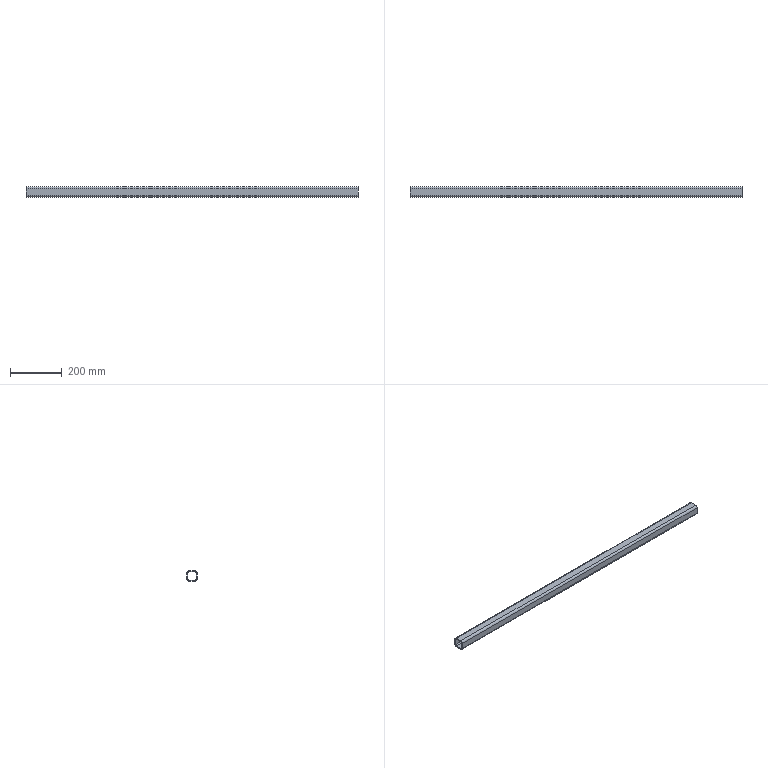Part | SolidWorks | features WeldMemberFeat 1, WeldmentFeature 1 | 1 solid | 18 faces | box 1280 x 40 x 40 mm | volume 684539 mm3 | plane 10 | cylinder 8 | commonest cylinder face diameters 8 x4 16 x4
STEP:
#1=CARTESIAN_POINT('',(-1000.,20.,12.));
#2=VERTEX_POINT('',#1);
#3=CARTESIAN_POINT('',(-1000.,12.,20.));
#4=VERTEX_POINT('',#3);
#5=CARTESIAN_POINT('',(-1000.,12.,12.));
#6=DIRECTION('',(1.,0.,0.));
#7=DIRECTION('',(0.,0.,-1.));
#8=AXIS2_PLACEMENT_3D('',#5,#6,#7);
#9=CIRCLE('',#8,8.);
#10=EDGE_CURVE('',#2,#4,#9,.T.);
#11=ORIENTED_EDGE('',*,*,#10,.T.);
#12=CARTESIAN_POINT('',(280.,12.,20.));
#13=VERTEX_POINT('',#12);
#14=CARTESIAN_POINT('',(280.,12.,20.));
#15=DIRECTION('',(-1.,0.,0.));
#16=VECTOR('',#15,1000.);
#17=LINE('',#14,#16);
#18=EDGE_CURVE('',#13,#4,#17,.T.);
#19=ORIENTED_EDGE('',*,*,#18,.F.);
#20=CARTESIAN_POINT('',(280.,20.,12.));
#21=VERTEX_POINT('',#20);
#22=CARTESIAN_POINT('',(280.,12.,12.));
#23=DIRECTION('',(1.,0.,0.));
#24=DIRECTION('',(0.,0.,-1.));
#25=AXIS2_PLACEMENT_3D('',#22,#23,#24);
#26=CIRCLE('',#25,8.);
#27=EDGE_CURVE('',#21,#13,#26,.T.);
#28=ORIENTED_EDGE('',*,*,#27,.F.);
#29=CARTESIAN_POINT('',(280.,20.,12.));
#30=DIRECTION('',(-1.,0.,0.));
#31=VECTOR('',#30,1000.);
#32=LINE('',#29,#31);
#33=EDGE_CURVE('',#21,#2,#32,.T.);
#34=ORIENTED_EDGE('',*,*,#33,.T.);
#35=EDGE_LOOP('',(#11,#19,#28,#34));
#36=FACE_OUTER_BOUND('',#35,.T.);
#37=CARTESIAN_POINT('',(280.,12.,12.));
#38=DIRECTION('',(-1.,0.,0.));
#39=DIRECTION('',(0.,0.,1.));
#40=AXIS2_PLACEMENT_3D('',#37,#38,#39);
#41=CYLINDRICAL_SURFACE('',#40,8.);
#42=ADVANCED_FACE('',(#36),#41,.T.);
#43=CARTESIAN_POINT('',(-1000.,-12.,20.));
#44=VERTEX_POINT('',#43);
#45=CARTESIAN_POINT('',(-1000.,12.,20.));
#46=DIRECTION('',(0.,-1.,0.));
#47=VECTOR('',#46,1000.);
#48=LINE('',#45,#47);
#49=EDGE_CURVE('',#4,#44,#48,.T.);
#50=ORIENTED_EDGE('',*,*,#49,.T.);
#51=CARTESIAN_POINT('',(280.,-12.,20.));
#52=VERTEX_POINT('',#51);
#53=CARTESIAN_POINT('',(280.,-12.,20.));
#54=DIRECTION('',(-1.,0.,0.));
#55=VECTOR('',#54,1000.);
#56=LINE('',#53,#55);
#57=EDGE_CURVE('',#52,#44,#56,.T.);
#58=ORIENTED_EDGE('',*,*,#57,.F.);
#59=CARTESIAN_POINT('',(280.,12.,20.));
#60=DIRECTION('',(0.,-1.,0.));
#61=VECTOR('',#60,1000.);
#62=LINE('',#59,#61);
#63=EDGE_CURVE('',#13,#52,#62,.T.);
#64=ORIENTED_EDGE('',*,*,#63,.F.);
#65=ORIENTED_EDGE('',*,*,#18,.T.);
#66=EDGE_LOOP('',(#50,#58,#64,#65));
#67=FACE_OUTER_BOUND('',#66,.T.);
#68=CARTESIAN_POINT('',(280.,12.,20.));
#69=DIRECTION('',(0.,0.,-1.));
#70=DIRECTION('',(-1.,0.,0.));
#71=AXIS2_PLACEMENT_3D('',#68,#69,#70);
#72=PLANE('',#71);
#73=ADVANCED_FACE('',(#67),#72,.F.);
#74=CARTESIAN_POINT('',(-1000.,-20.,12.));
#75=VERTEX_POINT('',#74);
#76=CARTESIAN_POINT('',(-1000.,-12.,12.));
#77=DIRECTION('',(1.,0.,0.));
#78=DIRECTION('',(0.,0.,-1.));
#79=AXIS2_PLACEMENT_3D('',#76,#77,#78);
#80=CIRCLE('',#79,8.);
#81=EDGE_CURVE('',#44,#75,#80,.T.);
#82=ORIENTED_EDGE('',*,*,#81,.T.);
#83=CARTESIAN_POINT('',(280.,-20.,12.));
#84=VERTEX_POINT('',#83);
#85=CARTESIAN_POINT('',(280.,-20.,12.));
#86=DIRECTION('',(-1.,0.,0.));
#87=VECTOR('',#86,1000.);
#88=LINE('',#85,#87);
#89=EDGE_CURVE('',#84,#75,#88,.T.);
#90=ORIENTED_EDGE('',*,*,#89,.F.);
#91=CARTESIAN_POINT('',(280.,-12.,12.));
#92=DIRECTION('',(1.,0.,0.));
#93=DIRECTION('',(0.,0.,-1.));
#94=AXIS2_PLACEMENT_3D('',#91,#92,#93);
#95=CIRCLE('',#94,8.);
#96=EDGE_CURVE('',#52,#84,#95,.T.);
#97=ORIENTED_EDGE('',*,*,#96,.F.);
#98=ORIENTED_EDGE('',*,*,#57,.T.);
#99=EDGE_LOOP('',(#82,#90,#97,#98));
#100=FACE_OUTER_BOUND('',#99,.T.);
#101=CARTESIAN_POINT('',(280.,-12.,12.));
#102=DIRECTION('',(-1.,0.,0.));
#103=DIRECTION('',(0.,0.,1.));
#104=AXIS2_PLACEMENT_3D('',#101,#102,#103);
#105=CYLINDRICAL_SURFACE('',#104,8.);
#106=ADVANCED_FACE('',(#100),#105,.T.);
#107=CARTESIAN_POINT('',(-1000.,-20.,-12.));
#108=VERTEX_POINT('',#107);
#109=CARTESIAN_POINT('',(-1000.,-20.,-12.));
#110=DIRECTION('',(0.,0.,-1.));
#111=VECTOR('',#110,1000.);
#112=LINE('',#109,#111);
#113=EDGE_CURVE('',#75,#108,#112,.T.);
#114=ORIENTED_EDGE('',*,*,#113,.T.);
#115=CARTESIAN_POINT('',(280.,-20.,-12.));
#116=VERTEX_POINT('',#115);
#117=CARTESIAN_POINT('',(280.,-20.,-12.));
#118=DIRECTION('',(-1.,0.,0.));
#119=VECTOR('',#118,1000.);
#120=LINE('',#117,#119);
#121=EDGE_CURVE('',#116,#108,#120,.T.);
#122=ORIENTED_EDGE('',*,*,#121,.F.);
#123=CARTESIAN_POINT('',(280.,-20.,-12.));
#124=DIRECTION('',(0.,0.,-1.));
#125=VECTOR('',#124,1000.);
#126=LINE('',#123,#125);
#127=EDGE_CURVE('',#84,#116,#126,.T.);
#128=ORIENTED_EDGE('',*,*,#127,.F.);
#129=ORIENTED_EDGE('',*,*,#89,.T.);
#130=EDGE_LOOP('',(#114,#122,#128,#129));
#131=FACE_OUTER_BOUND('',#130,.T.);
#132=CARTESIAN_POINT('',(280.,-20.,-12.));
#133=DIRECTION('',(0.,1.,0.));
#134=DIRECTION('',(0.,0.,1.));
#135=AXIS2_PLACEMENT_3D('',#132,#133,#134);
#136=PLANE('',#135);
#137=ADVANCED_FACE('',(#131),#136,.F.);
#138=CARTESIAN_POINT('',(-1000.,-12.,-20.));
#139=VERTEX_POINT('',#138);
#140=CARTESIAN_POINT('',(-1000.,-12.,-12.));
#141=DIRECTION('',(1.,0.,0.));
#142=DIRECTION('',(0.,0.,-1.));
#143=AXIS2_PLACEMENT_3D('',#140,#141,#142);
#144=CIRCLE('',#143,8.);
#145=EDGE_CURVE('',#108,#139,#144,.T.);
#146=ORIENTED_EDGE('',*,*,#145,.T.);
#147=CARTESIAN_POINT('',(280.,-12.,-20.));
#148=VERTEX_POINT('',#147);
#149=CARTESIAN_POINT('',(280.,-12.,-20.));
#150=DIRECTION('',(-1.,0.,0.));
#151=VECTOR('',#150,1000.);
#152=LINE('',#149,#151);
#153=EDGE_CURVE('',#148,#139,#152,.T.);
#154=ORIENTED_EDGE('',*,*,#153,.F.);
#155=CARTESIAN_POINT('',(280.,-12.,-12.));
#156=DIRECTION('',(1.,0.,0.));
#157=DIRECTION('',(0.,0.,-1.));
#158=AXIS2_PLACEMENT_3D('',#155,#156,#157);
#159=CIRCLE('',#158,8.);
#160=EDGE_CURVE('',#116,#148,#159,.T.);
#161=ORIENTED_EDGE('',*,*,#160,.F.);
#162=ORIENTED_EDGE('',*,*,#121,.T.);
#163=EDGE_LOOP('',(#146,#154,#161,#162));
#164=FACE_OUTER_BOUND('',#163,.T.);
#165=CARTESIAN_POINT('',(280.,-12.,-12.));
#166=DIRECTION('',(-1.,0.,0.));
#167=DIRECTION('',(0.,0.,1.));
#168=AXIS2_PLACEMENT_3D('',#165,#166,#167);
#169=CYLINDRICAL_SURFACE('',#168,8.);
#170=ADVANCED_FACE('',(#164),#169,.T.);
#171=CARTESIAN_POINT('',(-1000.,12.,-20.));
#172=VERTEX_POINT('',#171);
#173=CARTESIAN_POINT('',(-1000.,-12.,-20.));
#174=DIRECTION('',(0.,1.,0.));
#175=VECTOR('',#174,1000.);
#176=LINE('',#173,#175);
#177=EDGE_CURVE('',#139,#172,#176,.T.);
#178=ORIENTED_EDGE('',*,*,#177,.T.);
#179=CARTESIAN_POINT('',(280.,12.,-20.));
#180=VERTEX_POINT('',#179);
#181=CARTESIAN_POINT('',(280.,12.,-20.));
#182=DIRECTION('',(-1.,0.,0.));
#183=VECTOR('',#182,1000.);
#184=LINE('',#181,#183);
#185=EDGE_CURVE('',#180,#172,#184,.T.);
#186=ORIENTED_EDGE('',*,*,#185,.F.);
#187=CARTESIAN_POINT('',(280.,-12.,-20.));
#188=DIRECTION('',(0.,1.,0.));
#189=VECTOR('',#188,1000.);
#190=LINE('',#187,#189);
#191=EDGE_CURVE('',#148,#180,#190,.T.);
#192=ORIENTED_EDGE('',*,*,#191,.F.);
#193=ORIENTED_EDGE('',*,*,#153,.T.);
#194=EDGE_LOOP('',(#178,#186,#192,#193));
#195=FACE_OUTER_BOUND('',#194,.T.);
#196=CARTESIAN_POINT('',(280.,-12.,-20.));
#197=DIRECTION('',(0.,0.,1.));
#198=DIRECTION('',(1.,0.,0.));
#199=AXIS2_PLACEMENT_3D('',#196,#197,#198);
#200=PLANE('',#199);
#201=ADVANCED_FACE('',(#195),#200,.F.);
#202=CARTESIAN_POINT('',(-1000.,20.,-12.));
#203=VERTEX_POINT('',#202);
#204=CARTESIAN_POINT('',(-1000.,12.,-12.));
#205=DIRECTION('',(1.,0.,0.));
#206=DIRECTION('',(0.,0.,-1.));
#207=AXIS2_PLACEMENT_3D('',#204,#205,#206);
#208=CIRCLE('',#207,8.);
#209=EDGE_CURVE('',#172,#203,#208,.T.);
#210=ORIENTED_EDGE('',*,*,#209,.T.);
#211=CARTESIAN_POINT('',(280.,20.,-12.));
#212=VERTEX_POINT('',#211);
#213=CARTESIAN_POINT('',(280.,20.,-12.));
#214=DIRECTION('',(-1.,0.,0.));
#215=VECTOR('',#214,1000.);
#216=LINE('',#213,#215);
#217=EDGE_CURVE('',#212,#203,#216,.T.);
#218=ORIENTED_EDGE('',*,*,#217,.F.);
#219=CARTESIAN_POINT('',(280.,12.,-12.));
#220=DIRECTION('',(1.,0.,0.));
#221=DIRECTION('',(0.,0.,-1.));
#222=AXIS2_PLACEMENT_3D('',#219,#220,#221);
#223=CIRCLE('',#222,8.);
#224=EDGE_CURVE('',#180,#212,#223,.T.);
#225=ORIENTED_EDGE('',*,*,#224,.F.);
#226=ORIENTED_EDGE('',*,*,#185,.T.);
#227=EDGE_LOOP('',(#210,#218,#225,#226));
#228=FACE_OUTER_BOUND('',#227,.T.);
#229=CARTESIAN_POINT('',(280.,12.,-12.));
#230=DIRECTION('',(-1.,0.,0.));
#231=DIRECTION('',(0.,0.,1.));
#232=AXIS2_PLACEMENT_3D('',#229,#230,#231);
#233=CYLINDRICAL_SURFACE('',#232,8.);
#234=ADVANCED_FACE('',(#228),#233,.T.);
#235=CARTESIAN_POINT('',(-1000.,-12.,16.));
#236=VERTEX_POINT('',#235);
#237=CARTESIAN_POINT('',(-1000.,-16.,12.));
#238=VERTEX_POINT('',#237);
#239=CARTESIAN_POINT('',(-1000.,-12.,12.));
#240=DIRECTION('',(1.,0.,0.));
#241=DIRECTION('',(0.,0.,-1.));
#242=AXIS2_PLACEMENT_3D('',#239,#240,#241);
#243=CIRCLE('',#242,4.);
#244=EDGE_CURVE('',#236,#238,#243,.T.);
#245=ORIENTED_EDGE('',*,*,#244,.F.);
#246=CARTESIAN_POINT('',(280.,-12.,16.));
#247=VERTEX_POINT('',#246);
#248=CARTESIAN_POINT('',(280.,-12.,16.));
#249=DIRECTION('',(-1.,0.,0.));
#250=VECTOR('',#249,1000.);
#251=LINE('',#248,#250);
#252=EDGE_CURVE('',#247,#236,#251,.T.);
#253=ORIENTED_EDGE('',*,*,#252,.F.);
#254=CARTESIAN_POINT('',(280.,-16.,12.));
#255=VERTEX_POINT('',#254);
#256=CARTESIAN_POINT('',(280.,-12.,12.));
#257=DIRECTION('',(1.,0.,0.));
#258=DIRECTION('',(0.,0.,-1.));
#259=AXIS2_PLACEMENT_3D('',#256,#257,#258);
#260=CIRCLE('',#259,4.);
#261=EDGE_CURVE('',#247,#255,#260,.T.);
#262=ORIENTED_EDGE('',*,*,#261,.T.);
#263=CARTESIAN_POINT('',(280.,-16.,12.));
#264=DIRECTION('',(-1.,0.,0.));
#265=VECTOR('',#264,1000.);
#266=LINE('',#263,#265);
#267=EDGE_CURVE('',#255,#238,#266,.T.);
#268=ORIENTED_EDGE('',*,*,#267,.T.);
#269=EDGE_LOOP('',(#245,#253,#262,#268));
#270=FACE_OUTER_BOUND('',#269,.T.);
#271=CARTESIAN_POINT('',(280.,-12.,12.));
#272=DIRECTION('',(-1.,0.,0.));
#273=DIRECTION('',(0.,0.,1.));
#274=AXIS2_PLACEMENT_3D('',#271,#272,#273);
#275=CYLINDRICAL_SURFACE('',#274,4.);
#276=ADVANCED_FACE('',(#270),#275,.F.);
#277=CARTESIAN_POINT('',(-1000.,12.,16.));
#278=VERTEX_POINT('',#277);
#279=CARTESIAN_POINT('',(-1000.,12.,16.));
#280=DIRECTION('',(0.,-1.,0.));
#281=VECTOR('',#280,1000.);
#282=LINE('',#279,#281);
#283=EDGE_CURVE('',#278,#236,#282,.T.);
#284=ORIENTED_EDGE('',*,*,#283,.F.);
#285=CARTESIAN_POINT('',(280.,12.,16.));
#286=VERTEX_POINT('',#285);
#287=CARTESIAN_POINT('',(280.,12.,16.));
#288=DIRECTION('',(-1.,0.,0.));
#289=VECTOR('',#288,1000.);
#290=LINE('',#287,#289);
#291=EDGE_CURVE('',#286,#278,#290,.T.);
#292=ORIENTED_EDGE('',*,*,#291,.F.);
#293=CARTESIAN_POINT('',(280.,12.,16.));
#294=DIRECTION('',(0.,-1.,0.));
#295=VECTOR('',#294,1000.);
#296=LINE('',#293,#295);
#297=EDGE_CURVE('',#286,#247,#296,.T.);
#298=ORIENTED_EDGE('',*,*,#297,.T.);
#299=ORIENTED_EDGE('',*,*,#252,.T.);
#300=EDGE_LOOP('',(#284,#292,#298,#299));
#301=FACE_OUTER_BOUND('',#300,.T.);
#302=CARTESIAN_POINT('',(280.,12.,16.));
#303=DIRECTION('',(0.,0.,-1.));
#304=DIRECTION('',(-1.,0.,0.));
#305=AXIS2_PLACEMENT_3D('',#302,#303,#304);
#306=PLANE('',#305);
#307=ADVANCED_FACE('',(#301),#306,.T.);
#308=CARTESIAN_POINT('',(-1000.,16.,12.));
#309=VERTEX_POINT('',#308);
#310=CARTESIAN_POINT('',(-1000.,12.,12.));
#311=DIRECTION('',(1.,0.,0.));
#312=DIRECTION('',(0.,0.,-1.));
#313=AXIS2_PLACEMENT_3D('',#310,#311,#312);
#314=CIRCLE('',#313,4.);
#315=EDGE_CURVE('',#309,#278,#314,.T.);
#316=ORIENTED_EDGE('',*,*,#315,.F.);
#317=CARTESIAN_POINT('',(280.,16.,12.));
#318=VERTEX_POINT('',#317);
#319=CARTESIAN_POINT('',(280.,16.,12.));
#320=DIRECTION('',(-1.,0.,0.));
#321=VECTOR('',#320,1000.);
#322=LINE('',#319,#321);
#323=EDGE_CURVE('',#318,#309,#322,.T.);
#324=ORIENTED_EDGE('',*,*,#323,.F.);
#325=CARTESIAN_POINT('',(280.,12.,12.));
#326=DIRECTION('',(1.,0.,0.));
#327=DIRECTION('',(0.,0.,-1.));
#328=AXIS2_PLACEMENT_3D('',#325,#326,#327);
#329=CIRCLE('',#328,4.);
#330=EDGE_CURVE('',#318,#286,#329,.T.);
#331=ORIENTED_EDGE('',*,*,#330,.T.);
#332=ORIENTED_EDGE('',*,*,#291,.T.);
#333=EDGE_LOOP('',(#316,#324,#331,#332));
#334=FACE_OUTER_BOUND('',#333,.T.);
#335=CARTESIAN_POINT('',(280.,12.,12.));
#336=DIRECTION('',(-1.,0.,0.));
#337=DIRECTION('',(0.,0.,1.));
#338=AXIS2_PLACEMENT_3D('',#335,#336,#337);
#339=CYLINDRICAL_SURFACE('',#338,4.);
#340=ADVANCED_FACE('',(#334),#339,.F.);
#341=CARTESIAN_POINT('',(-1000.,16.,-12.));
#342=VERTEX_POINT('',#341);
#343=CARTESIAN_POINT('',(-1000.,16.,12.));
#344=DIRECTION('',(0.,0.,1.));
#345=VECTOR('',#344,1000.);
#346=LINE('',#343,#345);
#347=EDGE_CURVE('',#342,#309,#346,.T.);
#348=ORIENTED_EDGE('',*,*,#347,.F.);
#349=CARTESIAN_POINT('',(280.,16.,-12.));
#350=VERTEX_POINT('',#349);
#351=CARTESIAN_POINT('',(280.,16.,-12.));
#352=DIRECTION('',(-1.,0.,0.));
#353=VECTOR('',#352,1000.);
#354=LINE('',#351,#353);
#355=EDGE_CURVE('',#350,#342,#354,.T.);
#356=ORIENTED_EDGE('',*,*,#355,.F.);
#357=CARTESIAN_POINT('',(280.,16.,12.));
#358=DIRECTION('',(0.,0.,1.));
#359=VECTOR('',#358,1000.);
#360=LINE('',#357,#359);
#361=EDGE_CURVE('',#350,#318,#360,.T.);
#362=ORIENTED_EDGE('',*,*,#361,.T.);
#363=ORIENTED_EDGE('',*,*,#323,.T.);
#364=EDGE_LOOP('',(#348,#356,#362,#363));
#365=FACE_OUTER_BOUND('',#364,.T.);
#366=CARTESIAN_POINT('',(280.,16.,12.));
#367=DIRECTION('',(0.,-1.,0.));
#368=DIRECTION('',(0.,0.,-1.));
#369=AXIS2_PLACEMENT_3D('',#366,#367,#368);
#370=PLANE('',#369);
#371=ADVANCED_FACE('',(#365),#370,.T.);
#372=CARTESIAN_POINT('',(-1000.,12.,-16.));
#373=VERTEX_POINT('',#372);
#374=CARTESIAN_POINT('',(-1000.,12.,-12.));
#375=DIRECTION('',(1.,0.,0.));
#376=DIRECTION('',(0.,0.,-1.));
#377=AXIS2_PLACEMENT_3D('',#374,#375,#376);
#378=CIRCLE('',#377,4.);
#379=EDGE_CURVE('',#373,#342,#378,.T.);
#380=ORIENTED_EDGE('',*,*,#379,.F.);
#381=CARTESIAN_POINT('',(280.,12.,-16.));
#382=VERTEX_POINT('',#381);
#383=CARTESIAN_POINT('',(280.,12.,-16.));
#384=DIRECTION('',(-1.,0.,0.));
#385=VECTOR('',#384,1000.);
#386=LINE('',#383,#385);
#387=EDGE_CURVE('',#382,#373,#386,.T.);
#388=ORIENTED_EDGE('',*,*,#387,.F.);
#389=CARTESIAN_POINT('',(280.,12.,-12.));
#390=DIRECTION('',(1.,0.,0.));
#391=DIRECTION('',(0.,0.,-1.));
#392=AXIS2_PLACEMENT_3D('',#389,#390,#391);
#393=CIRCLE('',#392,4.);
#394=EDGE_CURVE('',#382,#350,#393,.T.);
#395=ORIENTED_EDGE('',*,*,#394,.T.);
#396=ORIENTED_EDGE('',*,*,#355,.T.);
#397=EDGE_LOOP('',(#380,#388,#395,#396));
#398=FACE_OUTER_BOUND('',#397,.T.);
#399=CARTESIAN_POINT('',(280.,12.,-12.));
#400=DIRECTION('',(-1.,0.,0.));
#401=DIRECTION('',(0.,0.,1.));
#402=AXIS2_PLACEMENT_3D('',#399,#400,#401);
#403=CYLINDRICAL_SURFACE('',#402,4.);
#404=ADVANCED_FACE('',(#398),#403,.F.);
#405=CARTESIAN_POINT('',(-1000.,-12.,-16.));
#406=VERTEX_POINT('',#405);
#407=CARTESIAN_POINT('',(-1000.,-12.,-16.));
#408=DIRECTION('',(0.,1.,0.));
#409=VECTOR('',#408,1000.);
#410=LINE('',#407,#409);
#411=EDGE_CURVE('',#406,#373,#410,.T.);
#412=ORIENTED_EDGE('',*,*,#411,.F.);
#413=CARTESIAN_POINT('',(280.,-12.,-16.));
#414=VERTEX_POINT('',#413);
#415=CARTESIAN_POINT('',(280.,-12.,-16.));
#416=DIRECTION('',(-1.,0.,0.));
#417=VECTOR('',#416,1000.);
#418=LINE('',#415,#417);
#419=EDGE_CURVE('',#414,#406,#418,.T.);
#420=ORIENTED_EDGE('',*,*,#419,.F.);
#421=CARTESIAN_POINT('',(280.,-12.,-16.));
#422=DIRECTION('',(0.,1.,0.));
#423=VECTOR('',#422,1000.);
#424=LINE('',#421,#423);
#425=EDGE_CURVE('',#414,#382,#424,.T.);
#426=ORIENTED_EDGE('',*,*,#425,.T.);
#427=ORIENTED_EDGE('',*,*,#387,.T.);
#428=EDGE_LOOP('',(#412,#420,#426,#427));
#429=FACE_OUTER_BOUND('',#428,.T.);
#430=CARTESIAN_POINT('',(280.,-12.,-16.));
#431=DIRECTION('',(0.,0.,1.));
#432=DIRECTION('',(1.,0.,0.));
#433=AXIS2_PLACEMENT_3D('',#430,#431,#432);
#434=PLANE('',#433);
#435=ADVANCED_FACE('',(#429),#434,.T.);
#436=CARTESIAN_POINT('',(-1000.,-16.,-12.));
#437=VERTEX_POINT('',#436);
#438=CARTESIAN_POINT('',(-1000.,-12.,-12.));
#439=DIRECTION('',(1.,0.,0.));
#440=DIRECTION('',(0.,0.,-1.));
#441=AXIS2_PLACEMENT_3D('',#438,#439,#440);
#442=CIRCLE('',#441,4.);
#443=EDGE_CURVE('',#437,#406,#442,.T.);
#444=ORIENTED_EDGE('',*,*,#443,.F.);
#445=CARTESIAN_POINT('',(280.,-16.,-12.));
#446=VERTEX_POINT('',#445);
#447=CARTESIAN_POINT('',(280.,-16.,-12.));
#448=DIRECTION('',(-1.,0.,0.));
#449=VECTOR('',#448,1000.);
#450=LINE('',#447,#449);
#451=EDGE_CURVE('',#446,#437,#450,.T.);
#452=ORIENTED_EDGE('',*,*,#451,.F.);
#453=CARTESIAN_POINT('',(280.,-12.,-12.));
#454=DIRECTION('',(1.,0.,0.));
#455=DIRECTION('',(0.,0.,-1.));
#456=AXIS2_PLACEMENT_3D('',#453,#454,#455);
#457=CIRCLE('',#456,4.);
#458=EDGE_CURVE('',#446,#414,#457,.T.);
#459=ORIENTED_EDGE('',*,*,#458,.T.);
#460=ORIENTED_EDGE('',*,*,#419,.T.);
#461=EDGE_LOOP('',(#444,#452,#459,#460));
#462=FACE_OUTER_BOUND('',#461,.T.);
#463=CARTESIAN_POINT('',(280.,-12.,-12.));
#464=DIRECTION('',(-1.,0.,0.));
#465=DIRECTION('',(0.,0.,1.));
#466=AXIS2_PLACEMENT_3D('',#463,#464,#465);
#467=CYLINDRICAL_SURFACE('',#466,4.);
#468=ADVANCED_FACE('',(#462),#467,.F.);
#469=CARTESIAN_POINT('',(-1000.,-16.,-12.));
#470=DIRECTION('',(0.,0.,-1.));
#471=VECTOR('',#470,1000.);
#472=LINE('',#469,#471);
#473=EDGE_CURVE('',#238,#437,#472,.T.);
#474=ORIENTED_EDGE('',*,*,#473,.F.);
#475=ORIENTED_EDGE('',*,*,#267,.F.);
#476=CARTESIAN_POINT('',(280.,-16.,-12.));
#477=DIRECTION('',(0.,0.,-1.));
#478=VECTOR('',#477,1000.);
#479=LINE('',#476,#478);
#480=EDGE_CURVE('',#255,#446,#479,.T.);
#481=ORIENTED_EDGE('',*,*,#480,.T.);
#482=ORIENTED_EDGE('',*,*,#451,.T.);
#483=EDGE_LOOP('',(#474,#475,#481,#482));
#484=FACE_OUTER_BOUND('',#483,.T.);
#485=CARTESIAN_POINT('',(280.,-16.,-12.));
#486=DIRECTION('',(0.,1.,0.));
#487=DIRECTION('',(0.,0.,1.));
#488=AXIS2_PLACEMENT_3D('',#485,#486,#487);
#489=PLANE('',#488);
#490=ADVANCED_FACE('',(#484),#489,.T.);
#491=CARTESIAN_POINT('',(-1000.,20.,12.));
#492=DIRECTION('',(0.,0.,1.));
#493=VECTOR('',#492,1000.);
#494=LINE('',#491,#493);
#495=EDGE_CURVE('',#203,#2,#494,.T.);
#496=ORIENTED_EDGE('',*,*,#495,.T.);
#497=ORIENTED_EDGE('',*,*,#33,.F.);
#498=CARTESIAN_POINT('',(280.,20.,12.));
#499=DIRECTION('',(0.,0.,1.));
#500=VECTOR('',#499,1000.);
#501=LINE('',#498,#500);
#502=EDGE_CURVE('',#212,#21,#501,.T.);
#503=ORIENTED_EDGE('',*,*,#502,.F.);
#504=ORIENTED_EDGE('',*,*,#217,.T.);
#505=EDGE_LOOP('',(#496,#497,#503,#504));
#506=FACE_OUTER_BOUND('',#505,.T.);
#507=CARTESIAN_POINT('',(280.,20.,12.));
#508=DIRECTION('',(0.,-1.,0.));
#509=DIRECTION('',(0.,0.,-1.));
#510=AXIS2_PLACEMENT_3D('',#507,#508,#509);
#511=PLANE('',#510);
#512=ADVANCED_FACE('',(#506),#511,.F.);
#513=ORIENTED_EDGE('',*,*,#261,.F.);
#514=ORIENTED_EDGE('',*,*,#297,.F.);
#515=ORIENTED_EDGE('',*,*,#330,.F.);
#516=ORIENTED_EDGE('',*,*,#361,.F.);
#517=ORIENTED_EDGE('',*,*,#394,.F.);
#518=ORIENTED_EDGE('',*,*,#425,.F.);
#519=ORIENTED_EDGE('',*,*,#458,.F.);
#520=ORIENTED_EDGE('',*,*,#480,.F.);
#521=EDGE_LOOP('',(#513,#514,#515,#516,#517,#518,#519,#520));
#522=FACE_BOUND('',#521,.T.);
#523=ORIENTED_EDGE('',*,*,#27,.T.);
#524=ORIENTED_EDGE('',*,*,#63,.T.);
#525=ORIENTED_EDGE('',*,*,#96,.T.);
#526=ORIENTED_EDGE('',*,*,#127,.T.);
#527=ORIENTED_EDGE('',*,*,#160,.T.);
#528=ORIENTED_EDGE('',*,*,#191,.T.);
#529=ORIENTED_EDGE('',*,*,#224,.T.);
#530=ORIENTED_EDGE('',*,*,#502,.T.);
#531=EDGE_LOOP('',(#523,#524,#525,#526,#527,#528,#529,#530));
#532=FACE_OUTER_BOUND('',#531,.T.);
#533=CARTESIAN_POINT('',(280.,12.,12.));
#534=DIRECTION('',(1.,0.,0.));
#535=DIRECTION('',(0.,0.,-1.));
#536=AXIS2_PLACEMENT_3D('',#533,#534,#535);
#537=PLANE('',#536);
#538=ADVANCED_FACE('',(#522,#532),#537,.T.);
#539=ORIENTED_EDGE('',*,*,#244,.T.);
#540=ORIENTED_EDGE('',*,*,#473,.T.);
#541=ORIENTED_EDGE('',*,*,#443,.T.);
#542=ORIENTED_EDGE('',*,*,#411,.T.);
#543=ORIENTED_EDGE('',*,*,#379,.T.);
#544=ORIENTED_EDGE('',*,*,#347,.T.);
#545=ORIENTED_EDGE('',*,*,#315,.T.);
#546=ORIENTED_EDGE('',*,*,#283,.T.);
#547=EDGE_LOOP('',(#539,#540,#541,#542,#543,#544,#545,#546));
#548=FACE_BOUND('',#547,.T.);
#549=ORIENTED_EDGE('',*,*,#10,.F.);
#550=ORIENTED_EDGE('',*,*,#495,.F.);
#551=ORIENTED_EDGE('',*,*,#209,.F.);
#552=ORIENTED_EDGE('',*,*,#177,.F.);
#553=ORIENTED_EDGE('',*,*,#145,.F.);
#554=ORIENTED_EDGE('',*,*,#113,.F.);
#555=ORIENTED_EDGE('',*,*,#81,.F.);
#556=ORIENTED_EDGE('',*,*,#49,.F.);
#557=EDGE_LOOP('',(#549,#550,#551,#552,#553,#554,#555,#556));
#558=FACE_OUTER_BOUND('',#557,.T.);
#559=CARTESIAN_POINT('',(-1000.,12.,12.));
#560=DIRECTION('',(1.,0.,0.));
#561=DIRECTION('',(0.,0.,-1.));
#562=AXIS2_PLACEMENT_3D('',#559,#560,#561);
#563=PLANE('',#562);
#564=ADVANCED_FACE('',(#548,#558),#563,.F.);
#565=CLOSED_SHELL('',(#42,#73,#106,#137,#170,#201,#234,#276,#307,#340,#371,#404,#435,#468,#490,#512,#538,#564));
#566=MANIFOLD_SOLID_BREP('',#565);
#567=CARTESIAN_POINT('',(0.,0.,0.));
#568=DIRECTION('',(0.,0.,1.));
#569=DIRECTION('',(1.,0.,0.));
#570=AXIS2_PLACEMENT_3D('',#567,#568,#569);
#571=(LENGTH_UNIT()NAMED_UNIT(*)SI_UNIT(.MILLI.,.METRE.));
#572=UNCERTAINTY_MEASURE_WITH_UNIT(LENGTH_MEASURE(0.00001),#571,'','');
#573=(NAMED_UNIT(*)PLANE_ANGLE_UNIT()SI_UNIT($,.RADIAN.));
#574=(NAMED_UNIT(*)SI_UNIT($,.STERADIAN.)SOLID_ANGLE_UNIT());
#575=(GEOMETRIC_REPRESENTATION_CONTEXT(3)GLOBAL_UNCERTAINTY_ASSIGNED_CONTEXT((#572))GLOBAL_UNIT_ASSIGNED_CONTEXT((#571,#573,#574))REPRESENTATION_CONTEXT('',''));
#576=ADVANCED_BREP_SHAPE_REPRESENTATION('',(#566,#570),#575);